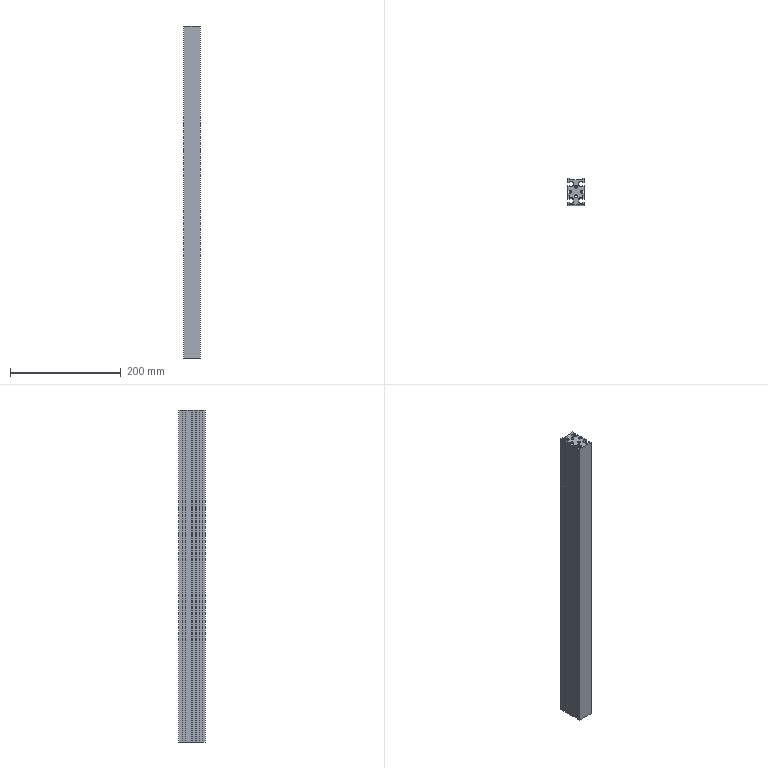Part | STEP file | Guide wheel mechanism revised.sldasm-Part-83 | 1 solid | 98 faces | box 30 x 48 x 600 mm | volume 562509 mm3 | plane 90 | cylinder 8 | commonest cylinder face diameters 1 x4 5 x4